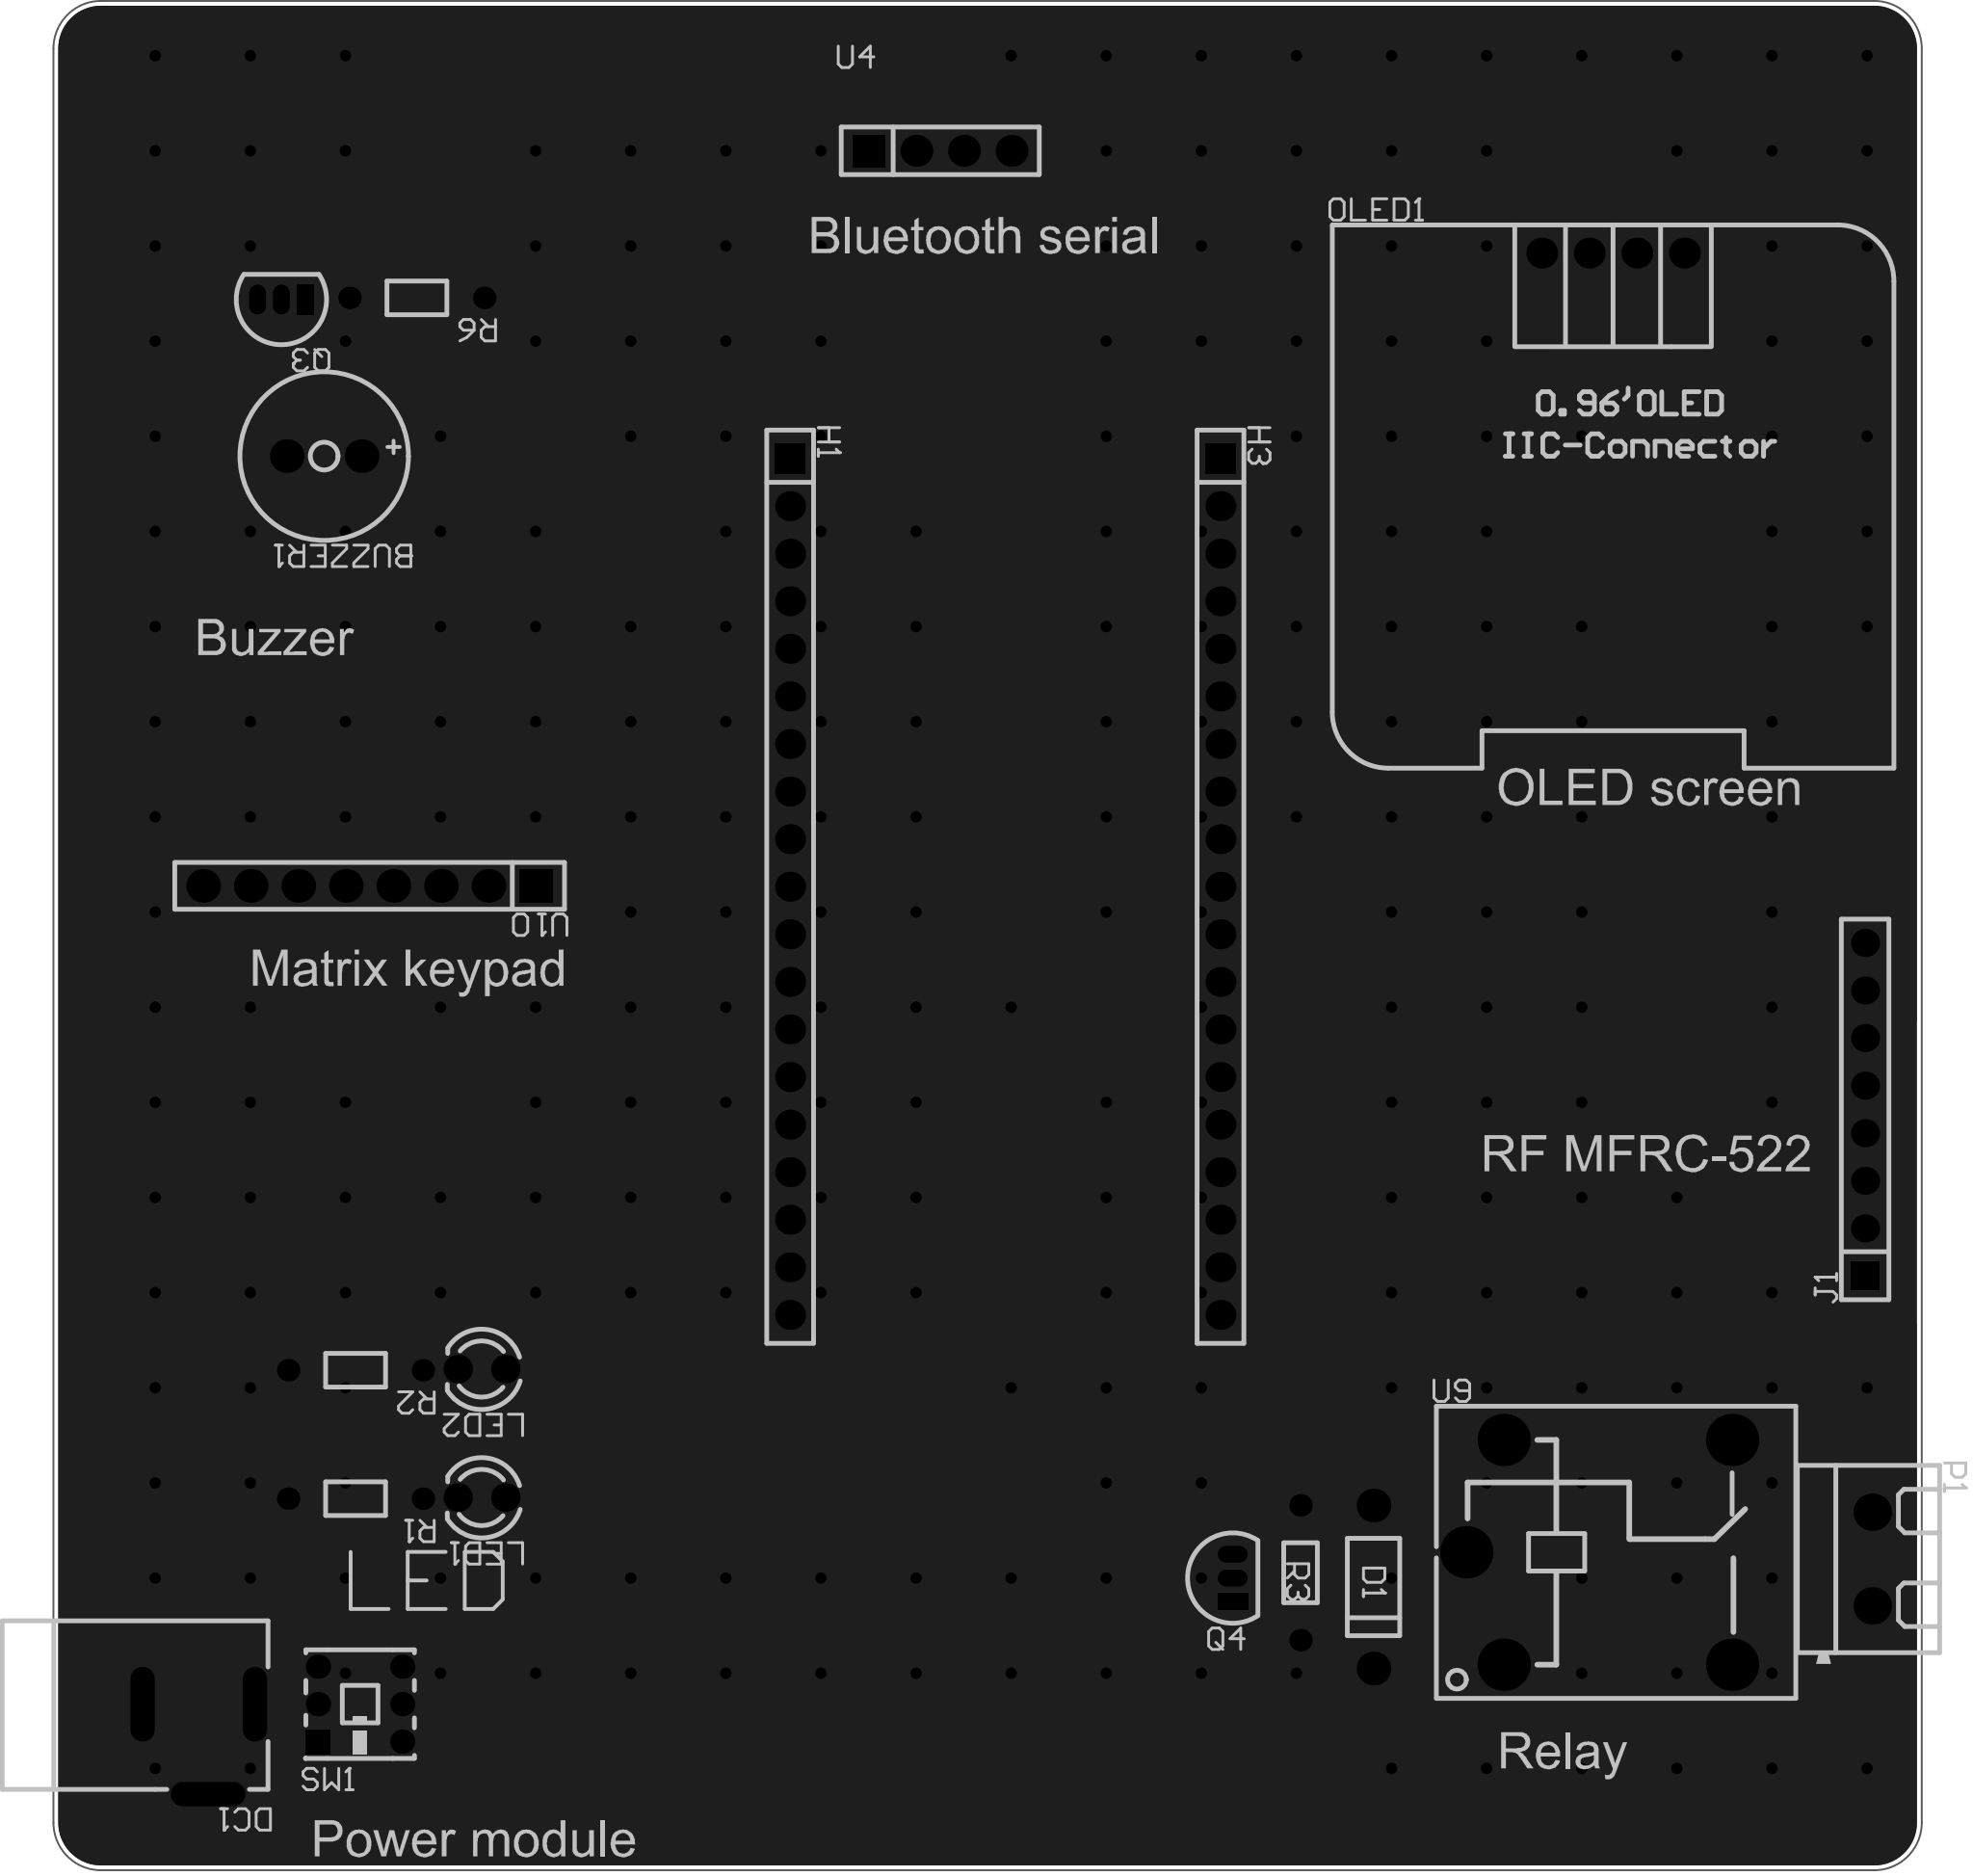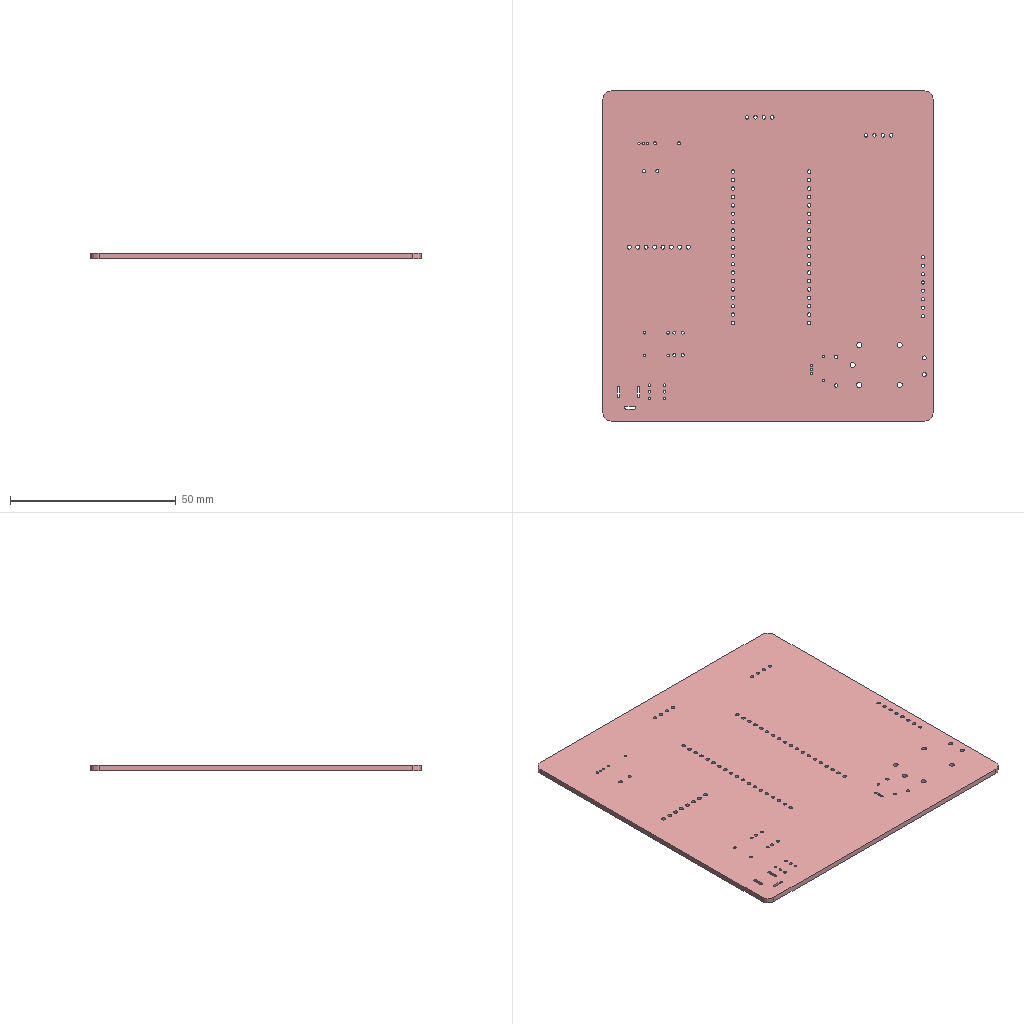Circuit board layout | Altium Designer | box 99.8 x 99.8 x 1.6 mm
Layer stack:
# Altium Designer layer stack of  (unit mm; dielectric type: 0 none, 1 core, 2 prepreg, 3 surface material)
index,name,kind,layer,copper_thickness_mm,dielectric_type,dielectric_thickness_mm,dielectric_material,dielectric_constant
0,Top Paste Mask Layer,other,,,,,,
1,Top Silkscreen Layer,other,,,,,,
2,Top Solder Mask Layer,dielectric,,,3,0.01,,3.3
3,Top Layer,copper,Top Layer,0.035,,,,
4,Dielectric1,dielectric,,,3,1.51,FR4,4.5
5,Bottom Layer,copper,Bottom Layer,0.035,,,,
6,Bottom Solder Mask Layer,dielectric,,,3,0.01,,3.3
7,Bottom Silkscreen Layer,other,,,,,,
8,Bottom Paste Mask Layer,other,,,,,,
# drill layer pairs: low layer,high layer
drill_pair,Top Layer,Bottom Layer
Part placement:
Designator,Comment,Layer,Footprint,Center-X(mm),Center-Y(mm),Rotation
BUZZER1,2.7kHz,TopLayer,BUZ-TH_BD9.0-P4.00-D0.6-FD,93.441,152.611,180
J1,,TopLayer,HDR-TH_8P-P2.54-V-M,175.753,117.729,90
U9,SRD-12VDC-SL-C,TopLayer,RELAY-TH_SRD-XXVDC-XL-C,161.55,94.086,0
U4,,TopLayer,HDR-TH_4P-P2.54-V-F,126.35,168.91,0
U10,,TopLayer,HDR-TH_8P-P2.54-V-F-1,95.87,129.667,180
SW1,5.8 WSPT,TopLayer,SW-TH_6P-L5.8-W5.8-P2.00-LS4.5-TL_K8-5851E-L1,95.362,85.979,90
R6,1K,TopLayer,Res_1/8W,98.394,161.057,180
Q3,,TopLayer,S8050_TO_92,91.155,160.967,180
D1,,TopLayer,DO_1N4007,149.495,92.232,90
Q4,,TopLayer,S8050_TO_92,141.971,92.71,90
R3,1K,TopLayer,Res_1/8W,145.595,92.994,270
H1,C2897382,TopLayer,HDR-TH_19P-P2.54-V-F,118.331,129.619,270
H3,C2897382,TopLayer,HDR-TH_19P-P2.54-V-F,141.318,129.619,270
LED1,,TopLayer,LED_TH-3mm,101.849,97.011,180
LED2,,TopLayer,LED_TH-3mm,101.849,103.869,180
OLED1,,TopLayer,0.96OLED_4P,162.291,163.449,0
R1,220Ω,TopLayer,Res_1/8W,95.118,96.948,180
R2,220Ω,TopLayer,Res_1/8W,95.118,103.806,180
DC1,,TopLayer,DC-2.0,86.741,83.574,180
P1,KF301-2P terminal block,TopLayer,CONN-TH_XY301V-A-5.0-2P,176.134,93.726,270
Pad and via stacks:
# Altium Designer via and pad stacks of  (unit mm). Each distinct definition once, with the count of objects using it.
# via: kind,start_layer,end_layer,hole_mm,diameter_mm,mode(0 simple;1 top-mid-bottom;2 full stack),diameter_per_layer,count,example_net
# pad: kind,layer,hole_mm,hole_type(0 round;1 square;2 slot),plating,top_size,top_shape(1 round;2 rect;3 octagon;9 rounded rect),mid_size,bottom_size,mode,footprint,size_per_layer,count,example
pad,Multi-Layer,1,0,plated,1.8x1.8,1,1.8x1.8,1.8x1.8,0,BUZ-TH_BD9.0-P4.00-D0.6-FD,,2,BUZZER1.1
pad,Multi-Layer,1,0,plated,1.5x1.5,2,1.5x1.5,1.5x1.5,0,HDR-TH_8P-P2.54-V-M,,1,J1.1
pad,Multi-Layer,1,0,plated,1.5x1.5,1,1.5x1.5,1.5x1.5,0,HDR-TH_8P-P2.54-V-M,,7,J1.2
pad,Multi-Layer,1.524,0,plated,2.794x2.794,1,2.794x2.794,2.794x2.794,0,RELAY-TH_SRD-XXVDC-XL-C,,5,U9.2
pad,Multi-Layer,1.1,0,plated,1.7x1.7,2,1.7x1.7,1.7x1.7,0,HDR-TH_4P-P2.54-V-F,,1,U4.1
pad,Multi-Layer,1.1,0,plated,1.7x1.7,1,1.7x1.7,1.7x1.7,0,HDR-TH_4P-P2.54-V-F,,3,U4.2
pad,Multi-Layer,1.2,0,plated,1.8x1.8,2,1.8x1.8,1.8x1.8,0,HDR-TH_8P-P2.54-V-F-1,,1,U10.1
pad,Multi-Layer,1.2,0,plated,1.8x1.8,1,1.8x1.8,1.8x1.8,0,HDR-TH_8P-P2.54-V-F-1,,7,U10.2
pad,Multi-Layer,0.8,0,plated,1.3x1.3,2,1.3x1.3,1.3x1.3,0,SW-TH_6P-L5.8-W5.8-P2.00-LS4.5-TL_K8-5851E-L1,,1,SW1.1
pad,Multi-Layer,0.8,0,plated,1.3x1.3,1,1.3x1.3,1.3x1.3,0,SW-TH_6P-L5.8-W5.8-P2.00-LS4.5-TL_K8-5851E-L1,,5,SW1.2
pad,Multi-Layer,0.8001,0,plated,1.199x1.199,1,1.199x1.199,1.199x1.199,0,Res_1/8W,,8,R6.1
pad,Multi-Layer,0.701,0,plated,0.8992x1.6,2,0.8992x1.6,0.8992x1.6,0,S8050_TO_92,,2,Q3.1
pad,Multi-Layer,0.701,0,plated,0.8992x1.6,1,0.8992x1.6,0.8992x1.6,0,S8050_TO_92,,4,Q3.2
pad,Multi-Layer,1,0,plated,1.8x1.8,1,1.8x1.8,1.8x1.8,0,DO_1N4007,,2,D1.1
pad,Multi-Layer,1.05,0,plated,1.6x1.6,1,1.6x1.6,1.6x1.6,0,HDR-TH_19P-P2.54-V-F,,36,H1.19
pad,Multi-Layer,1.05,0,plated,1.6x1.6,2,1.6x1.6,1.6x1.6,0,HDR-TH_19P-P2.54-V-F,,2,H1.1
pad,Multi-Layer,0.9144,0,plated,1.524x1.524,1,1.524x1.524,1.524x1.524,0,LED_TH-3mm,,4,LED1.1
pad,Multi-Layer,1,0,plated,1.65x1.65,1,1.65x1.65,1.65x1.65,0,0.96OLED_4P,,4,OLED1.4
pad,Multi-Layer,0.8001,2,plated,4x1.3,1,4x1.3,4x1.3,0,DC-2.0,,3,DC1.2
pad,Multi-Layer,1.2,0,plated,2x2,1,2x2,2x2,0,CONN-TH_XY301V-A-5.0-2P,,2,P1.1
via,Top Layer,Bottom Layer,0.3048,0.61,0,,259,GND
Copper pours:
name,layer,net,type(0 solid;1 hatched;2 none)
Top Layer-GND,Top Layer,GND,0
Bottom Layer-GND,Bottom Layer,GND,0